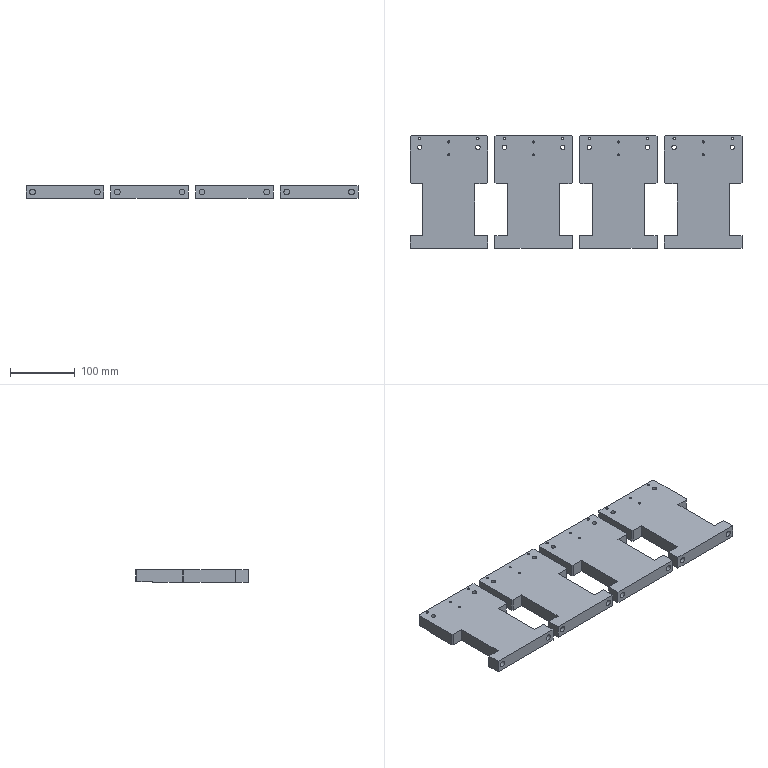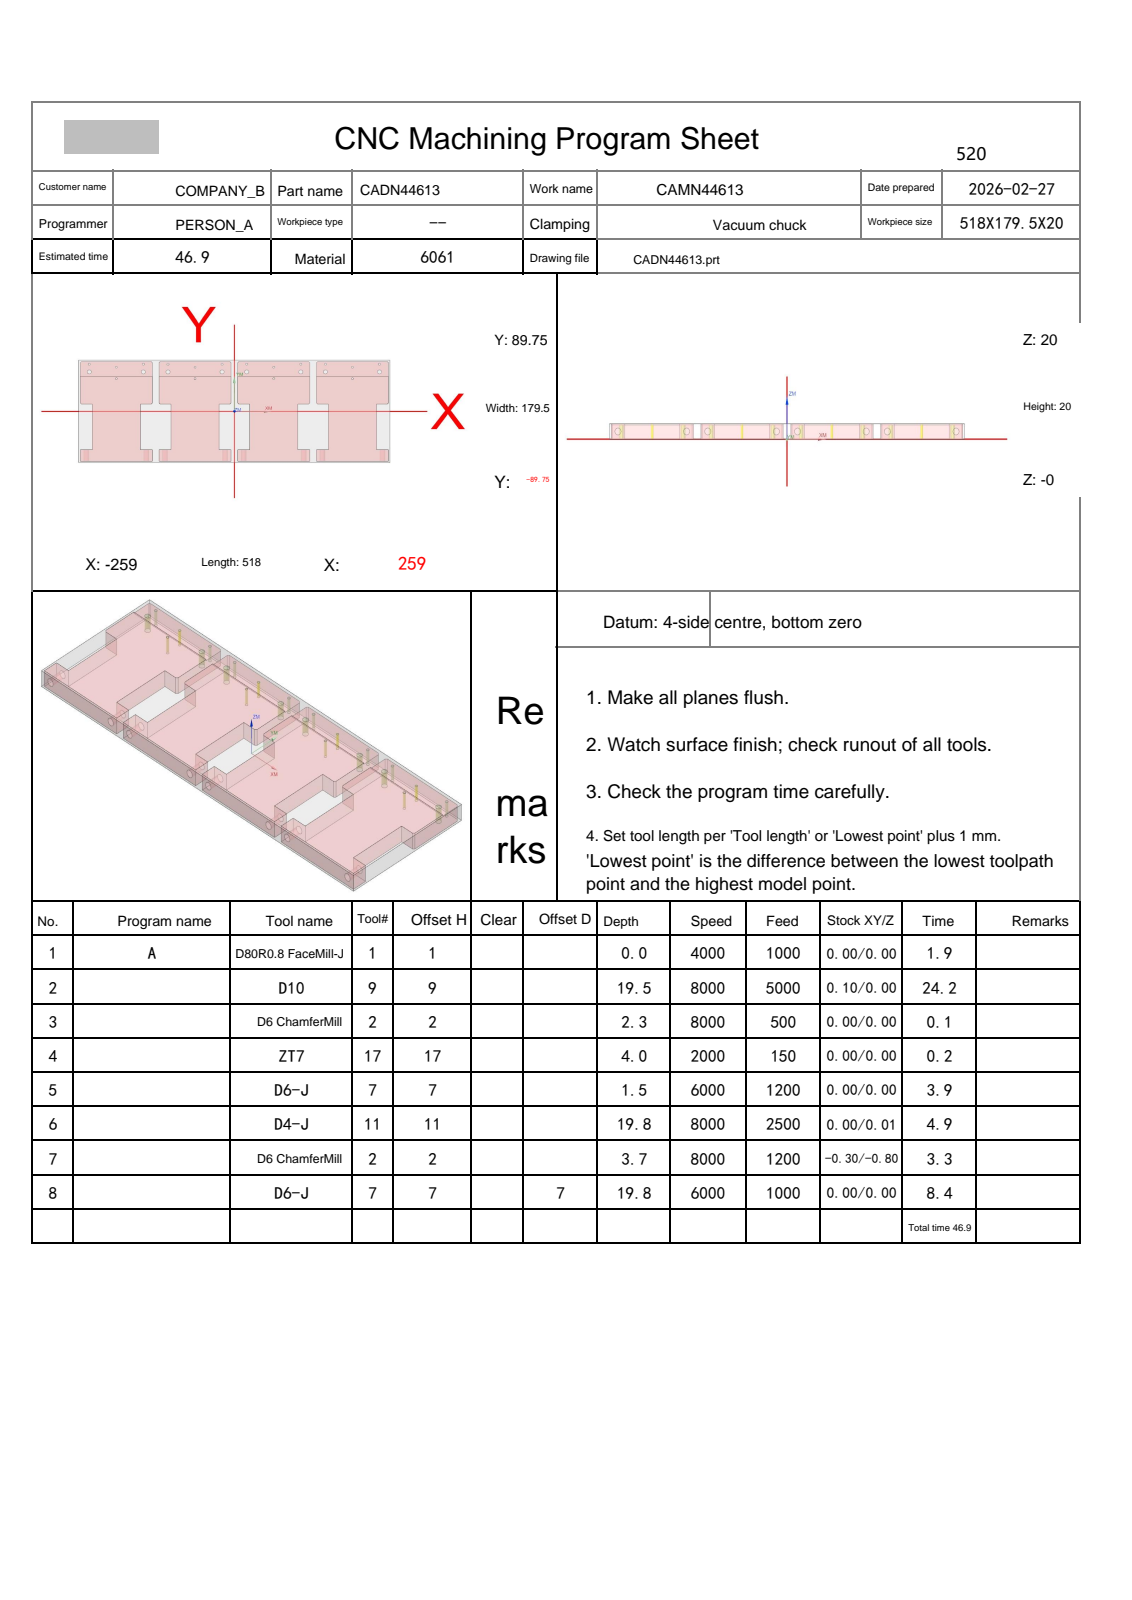NC program | NX | posted by the shop | part box 513 x 174.5 x 20 mm
Lines 41 to 1049 of 36838:
N2 T09 M06
(D10  D=10. R=0. H=09 ce=0.10 di=0.10)
G00 G90 G54 X-159.584 Y81.25 M03 S8000
G43 H09 Z50.
M08
Z20.5
G01 X-196.5 Z19.533 F4500.
X-250.5
Y73.2
X-142.5
Y81.25
X-196.5
Y88.25
X-254.914
X-257.5 Y85.664
Y66.2
X-135.5
Y85.664
X-138.086 Y88.25
X-196.5
X-197.
Z20.033
G00 Z20.5
X-159.584 Y81.25
Z20.033
G01 X-196.5 Z19.067
X-250.5
Y73.2
X-142.5
Y81.25
X-196.5
Y88.25
X-254.914
X-257.5 Y85.664
Y66.2
X-135.5
Y85.664
X-138.086 Y88.25
X-196.5
X-197.
Z19.567
G00 Z20.033
X-159.584 Y81.25
Z19.567
G01 X-196.5 Z18.6
X-250.5
Y73.2
X-142.5
Y81.25
X-196.5
Y88.25
X-254.914
X-257.5 Y85.664
Y66.2
X-135.5
Y85.664
X-138.086 Y88.25
X-196.5
X-197.
Z19.1
G00 Z50.
X-28.584 Y81.25
Z20.5
G01 X-65.5 Z19.533
X-119.5
Y73.2
X-11.5
Y81.25
X-65.5
Y88.25
X-123.914
X-126.5 Y85.664
Y66.2
X-4.5
Y85.664
X-7.086 Y88.25
X-65.5
X-66.
Z20.033
G00 Z20.5
X-28.584 Y81.25
Z20.033
G01 X-65.5 Z19.067
X-119.5
Y73.2
X-11.5
Y81.25
X-65.5
Y88.25
X-123.914
X-126.5 Y85.664
Y66.2
X-4.5
Y85.664
X-7.086 Y88.25
X-65.5
X-66.
Z19.567
G00 Z20.033
X-28.584 Y81.25
Z19.567
G01 X-65.5 Z18.6
X-119.5
Y73.2
X-11.5
Y81.25
X-65.5
Y88.25
X-123.914
X-126.5 Y85.664
Y66.2
X-4.5
Y85.664
X-7.086 Y88.25
X-65.5
X-66.
Z19.1
G00 Z50.
X102.416 Y81.25
Z20.5
G01 X65.5 Z19.533
X11.5
Y73.2
X119.5
Y81.25
X65.5
Y88.25
X7.086
X4.5 Y85.664
Y66.2
X126.5
Y85.664
X123.914 Y88.25
X65.5
X65.
Z20.033
G00 Z20.5
X102.416 Y81.25
Z20.033
G01 X65.5 Z19.067
X11.5
Y73.2
X119.5
Y81.25
X65.5
Y88.25
X7.086
X4.5 Y85.664
Y66.2
X126.5
Y85.664
X123.914 Y88.25
X65.5
X65.
Z19.567
G00 Z20.033
X102.416 Y81.25
Z19.567
G01 X65.5 Z18.6
X11.5
Y73.2
X119.5
Y81.25
X65.5
Y88.25
X7.086
X4.5 Y85.664
Y66.2
X126.5
Y85.664
X123.914 Y88.25
X65.5
X65.
Z19.1
G00 Z50.
X233.416 Y81.25
Z20.5
G01 X196.5 Z19.533
X142.5
Y73.2
X250.5
Y81.25
X196.5
Y88.25
X138.086
X135.5 Y85.664
Y66.2
X257.5
Y85.664
X254.914 Y88.25
X196.5
X196.
Z20.033
G00 Z20.5
X233.416 Y81.25
Z20.033
G01 X196.5 Z19.067
X142.5
Y73.2
X250.5
Y81.25
X196.5
Y88.25
X138.086
X135.5 Y85.664
Y66.2
X257.5
Y85.664
X254.914 Y88.25
X196.5
X196.
Z19.567
G00 Z20.033
X233.416 Y81.25
Z19.567
G01 X196.5 Z18.6
X142.5
Y73.2
X250.5
Y81.25
X196.5
Y88.25
X138.086
X135.5 Y85.664
Y66.2
X257.5
Y85.664
X254.914 Y88.25
X196.5
X196.
Z19.1
G00 Z50.
G00 G90 X196.5 Y-92.35 M03 S8000
Z50.
Z20.5
G01 X136.5 Z20.456 F5000.
G02 X131.4 Y-87.25 Z20.451 I0.0 J5.1
G01 Y-67.25 Z20.436
G02 X136.5 Y-62.15 Z20.43 I5.1 J0.0
G01 X151.4 Z20.419
Y7.65 Z20.369
X138.5 Z20.359
G02 X134.894 Y9.144 Z20.356 I0.0 J5.1
G01 X132.894 Y11.144 Z20.354
G02 X131.4 Y14.75 Z20.351 I3.606 J3.606
G01 Y85.25 Z20.3
G02 X132.894 Y88.856 Z20.297 I5.1 J0.0
G01 X134.894 Y90.856 Z20.295
G02 X138.5 Y92.35 Z20.292 I3.606 J-3.606
G01 X254.5 Z20.208
G02 X258.106 Y90.856 Z20.205 I0.0 J-5.1
G01 X260.106 Y88.856 Z20.203
G02 X261.6 Y85.25 Z20.2 I-3.606 J-3.606
G01 Y14.75 Z20.149
G02 X260.106 Y11.144 Z20.146 I-5.1 J0.0
G01 X258.106 Y9.144 Z20.144
G02 X254.5 Y7.65 Z20.141 I-3.606 J3.606
G01 X241.6 Z20.131
Y-62.15 Z20.081
X256.5 Z20.07
G02 X261.6 Y-67.25 Z20.064 I0.0 J-5.1
G01 Y-87.25 Z20.049
G02 X256.5 Y-92.35 Z20.044 I-5.1 J0.0
G01 X136.5 Z19.956
G02 X131.4 Y-87.25 Z19.951 I0.0 J5.1
G01 Y-67.25 Z19.936
G02 X136.5 Y-62.15 Z19.93 I5.1 J0.0
G01 X151.4 Z19.919
Y7.65 Z19.869
X138.5 Z19.859
G02 X134.894 Y9.144 Z19.856 I0.0 J5.1
G01 X132.894 Y11.144 Z19.854
G02 X131.4 Y14.75 Z19.851 I3.606 J3.606
G01 Y85.25 Z19.8
G02 X132.894 Y88.856 Z19.797 I5.1 J0.0
G01 X134.894 Y90.856 Z19.795
G02 X138.5 Y92.35 Z19.792 I3.606 J-3.606
G01 X254.5 Z19.708
G02 X258.106 Y90.856 Z19.705 I0.0 J-5.1
G01 X260.106 Y88.856 Z19.703
G02 X261.6 Y85.25 Z19.7 I-3.606 J-3.606
G01 Y14.75 Z19.649
G02 X260.106 Y11.144 Z19.646 I-5.1 J0.0
G01 X258.106 Y9.144 Z19.644
G02 X254.5 Y7.65 Z19.641 I-3.606 J3.606
G01 X241.6 Z19.631
Y-62.15 Z19.581
X256.5 Z19.57
G02 X261.6 Y-67.25 Z19.564 I0.0 J-5.1
G01 Y-87.25 Z19.549
G02 X256.5 Y-92.35 Z19.544 I-5.1 J0.0
G01 X136.5 Z19.456
G02 X131.4 Y-87.25 Z19.451 I0.0 J5.1
G01 Y-67.25 Z19.436
G02 X136.5 Y-62.15 Z19.43 I5.1 J0.0
G01 X151.4 Z19.419
Y7.65 Z19.369
X138.5 Z19.359
G02 X134.894 Y9.144 Z19.356 I0.0 J5.1
G01 X132.894 Y11.144 Z19.354
G02 X131.4 Y14.75 Z19.351 I3.606 J3.606
G01 Y85.25 Z19.3
G02 X132.894 Y88.856 Z19.297 I5.1 J0.0
G01 X134.894 Y90.856 Z19.295
G02 X138.5 Y92.35 Z19.292 I3.606 J-3.606
G01 X254.5 Z19.208
G02 X258.106 Y90.856 Z19.205 I0.0 J-5.1
G01 X260.106 Y88.856 Z19.203
G02 X261.6 Y85.25 Z19.2 I-3.606 J-3.606
G01 Y14.75 Z19.149
G02 X260.106 Y11.144 Z19.146 I-5.1 J0.0
G01 X258.106 Y9.144 Z19.144
G02 X254.5 Y7.65 Z19.141 I-3.606 J3.606
G01 X241.6 Z19.131
Y-62.15 Z19.081
X256.5 Z19.07
G02 X261.6 Y-67.25 Z19.064 I0.0 J-5.1
G01 Y-87.25 Z19.049
G02 X256.5 Y-92.35 Z19.044 I-5.1 J0.0
G01 X136.5 Z18.956
G02 X131.4 Y-87.25 Z18.951 I0.0 J5.1
G01 Y-67.25 Z18.936
G02 X136.5 Y-62.15 Z18.93 I5.1 J0.0
G01 X151.4 Z18.919
Y7.65 Z18.869
X138.5 Z18.859
G02 X134.894 Y9.144 Z18.856 I0.0 J5.1
G01 X132.894 Y11.144 Z18.854
G02 X131.4 Y14.75 Z18.851 I3.606 J3.606
G01 Y85.25 Z18.8
G02 X132.894 Y88.856 Z18.797 I5.1 J0.0
G01 X134.894 Y90.856 Z18.795
G02 X138.5 Y92.35 Z18.792 I3.606 J-3.606
G01 X254.5 Z18.708
G02 X258.106 Y90.856 Z18.705 I0.0 J-5.1
G01 X260.106 Y88.856 Z18.703
G02 X261.6 Y85.25 Z18.7 I-3.606 J-3.606
G01 Y14.75 Z18.649
G02 X260.106 Y11.144 Z18.646 I-5.1 J0.0
G01 X258.106 Y9.144 Z18.644
G02 X254.5 Y7.65 Z18.641 I-3.606 J3.606
G01 X241.6 Z18.631
Y-62.15 Z18.581
X256.5 Z18.57
G02 X261.6 Y-67.25 Z18.564 I0.0 J-5.1
G01 Y-87.25 Z18.549
G02 X256.5 Y-92.35 Z18.544 I-5.1 J0.0
G01 X136.5 Z18.456
G02 X131.4 Y-87.25 Z18.451 I0.0 J5.1
G01 Y-67.25 Z18.436
G02 X136.5 Y-62.15 Z18.43 I5.1 J0.0
G01 X151.4 Z18.419
Y7.65 Z18.369
X138.5 Z18.359
G02 X134.894 Y9.144 Z18.356 I0.0 J5.1
G01 X132.894 Y11.144 Z18.354
G02 X131.4 Y14.75 Z18.351 I3.606 J3.606
G01 Y85.25 Z18.3
G02 X132.894 Y88.856 Z18.297 I5.1 J0.0
G01 X134.894 Y90.856 Z18.295
G02 X138.5 Y92.35 Z18.292 I3.606 J-3.606
G01 X254.5 Z18.208
G02 X258.106 Y90.856 Z18.205 I0.0 J-5.1
G01 X260.106 Y88.856 Z18.203
G02 X261.6 Y85.25 Z18.2 I-3.606 J-3.606
G01 Y14.75 Z18.149
G02 X260.106 Y11.144 Z18.146 I-5.1 J0.0
G01 X258.106 Y9.144 Z18.144
G02 X254.5 Y7.65 Z18.141 I-3.606 J3.606
G01 X241.6 Z18.131
Y-62.15 Z18.081
X256.5 Z18.07
G02 X261.6 Y-67.25 Z18.064 I0.0 J-5.1
G01 Y-87.25 Z18.049
G02 X256.5 Y-92.35 Z18.044 I-5.1 J0.0
G01 X136.5 Z17.956
G02 X131.4 Y-87.25 Z17.951 I0.0 J5.1
G01 Y-67.25 Z17.936
G02 X136.5 Y-62.15 Z17.93 I5.1 J0.0
G01 X151.4 Z17.919
Y7.65 Z17.869
X138.5 Z17.859
G02 X134.894 Y9.144 Z17.856 I0.0 J5.1
G01 X132.894 Y11.144 Z17.854
G02 X131.4 Y14.75 Z17.851 I3.606 J3.606
G01 Y85.25 Z17.8
G02 X132.894 Y88.856 Z17.797 I5.1 J0.0
G01 X134.894 Y90.856 Z17.795
G02 X138.5 Y92.35 Z17.792 I3.606 J-3.606
G01 X254.5 Z17.708
G02 X258.106 Y90.856 Z17.705 I0.0 J-5.1
G01 X260.106 Y88.856 Z17.703
G02 X261.6 Y85.25 Z17.7 I-3.606 J-3.606
G01 Y14.75 Z17.649
G02 X260.106 Y11.144 Z17.646 I-5.1 J0.0
G01 X258.106 Y9.144 Z17.644
G02 X254.5 Y7.65 Z17.641 I-3.606 J3.606
G01 X241.6 Z17.631
Y-62.15 Z17.581
X256.5 Z17.57
G02 X261.6 Y-67.25 Z17.564 I0.0 J-5.1
G01 Y-87.25 Z17.549
G02 X256.5 Y-92.35 Z17.544 I-5.1 J0.0
G01 X136.5 Z17.456
G02 X131.4 Y-87.25 Z17.451 I0.0 J5.1
G01 Y-67.25 Z17.436
G02 X136.5 Y-62.15 Z17.43 I5.1 J0.0
G01 X151.4 Z17.419
Y7.65 Z17.369
X138.5 Z17.359
G02 X134.894 Y9.144 Z17.356 I0.0 J5.1
G01 X132.894 Y11.144 Z17.354
G02 X131.4 Y14.75 Z17.351 I3.606 J3.606
G01 Y85.25 Z17.3
G02 X132.894 Y88.856 Z17.297 I5.1 J0.0
G01 X134.894 Y90.856 Z17.295
G02 X138.5 Y92.35 Z17.292 I3.606 J-3.606
G01 X254.5 Z17.208
G02 X258.106 Y90.856 Z17.205 I0.0 J-5.1
G01 X260.106 Y88.856 Z17.203
G02 X261.6 Y85.25 Z17.2 I-3.606 J-3.606
G01 Y14.75 Z17.149
G02 X260.106 Y11.144 Z17.146 I-5.1 J0.0
G01 X258.106 Y9.144 Z17.144
G02 X254.5 Y7.65 Z17.141 I-3.606 J3.606
G01 X241.6 Z17.131
Y-62.15 Z17.081
X256.5 Z17.07
G02 X261.6 Y-67.25 Z17.064 I0.0 J-5.1
G01 Y-87.25 Z17.049
G02 X256.5 Y-92.35 Z17.044 I-5.1 J0.0
G01 X136.5 Z16.956
G02 X131.4 Y-87.25 Z16.951 I0.0 J5.1
G01 Y-67.25 Z16.936
G02 X136.5 Y-62.15 Z16.93 I5.1 J0.0
G01 X151.4 Z16.919
Y7.65 Z16.869
X138.5 Z16.859
G02 X134.894 Y9.144 Z16.856 I0.0 J5.1
G01 X132.894 Y11.144 Z16.854
G02 X131.4 Y14.75 Z16.851 I3.606 J3.606
G01 Y85.25 Z16.8
G02 X132.894 Y88.856 Z16.797 I5.1 J0.0
G01 X134.894 Y90.856 Z16.795
G02 X138.5 Y92.35 Z16.792 I3.606 J-3.606
G01 X254.5 Z16.708
G02 X258.106 Y90.856 Z16.705 I0.0 J-5.1
G01 X260.106 Y88.856 Z16.703
G02 X261.6 Y85.25 Z16.7 I-3.606 J-3.606
G01 Y14.75 Z16.649
G02 X260.106 Y11.144 Z16.646 I-5.1 J0.0
G01 X258.106 Y9.144 Z16.644
G02 X254.5 Y7.65 Z16.641 I-3.606 J3.606
G01 X241.6 Z16.631
Y-62.15 Z16.581
X256.5 Z16.57
G02 X261.6 Y-67.25 Z16.564 I0.0 J-5.1
G01 Y-87.25 Z16.549
G02 X256.5 Y-92.35 Z16.544 I-5.1 J0.0
G01 X136.5 Z16.456
G02 X131.4 Y-87.25 Z16.451 I0.0 J5.1
G01 Y-67.25 Z16.436
G02 X136.5 Y-62.15 Z16.43 I5.1 J0.0
G01 X151.4 Z16.419
Y7.65 Z16.369
X138.5 Z16.359
G02 X134.894 Y9.144 Z16.356 I0.0 J5.1
G01 X132.894 Y11.144 Z16.354
G02 X131.4 Y14.75 Z16.351 I3.606 J3.606
G01 Y85.25 Z16.3
G02 X132.894 Y88.856 Z16.297 I5.1 J0.0
G01 X134.894 Y90.856 Z16.295
G02 X138.5 Y92.35 Z16.292 I3.606 J-3.606
G01 X254.5 Z16.208
G02 X258.106 Y90.856 Z16.205 I0.0 J-5.1
G01 X260.106 Y88.856 Z16.203
G02 X261.6 Y85.25 Z16.2 I-3.606 J-3.606
G01 Y14.75 Z16.149
G02 X260.106 Y11.144 Z16.146 I-5.1 J0.0
G01 X258.106 Y9.144 Z16.144
G02 X254.5 Y7.65 Z16.141 I-3.606 J3.606
G01 X241.6 Z16.131
Y-62.15 Z16.081
X256.5 Z16.07
G02 X261.6 Y-67.25 Z16.064 I0.0 J-5.1
G01 Y-87.25 Z16.049
G02 X256.5 Y-92.35 Z16.044 I-5.1 J0.0
G01 X136.5 Z15.956
G02 X131.4 Y-87.25 Z15.951 I0.0 J5.1
G01 Y-67.25 Z15.936
G02 X136.5 Y-62.15 Z15.93 I5.1 J0.0
G01 X151.4 Z15.919
Y7.65 Z15.869
X138.5 Z15.859
G02 X134.894 Y9.144 Z15.856 I0.0 J5.1
G01 X132.894 Y11.144 Z15.854
G02 X131.4 Y14.75 Z15.851 I3.606 J3.606
G01 Y85.25 Z15.8
G02 X132.894 Y88.856 Z15.797 I5.1 J0.0
G01 X134.894 Y90.856 Z15.795
G02 X138.5 Y92.35 Z15.792 I3.606 J-3.606
G01 X254.5 Z15.708
G02 X258.106 Y90.856 Z15.705 I0.0 J-5.1
G01 X260.106 Y88.856 Z15.703
G02 X261.6 Y85.25 Z15.7 I-3.606 J-3.606
G01 Y14.75 Z15.649
G02 X260.106 Y11.144 Z15.646 I-5.1 J0.0
G01 X258.106 Y9.144 Z15.644
G02 X254.5 Y7.65 Z15.641 I-3.606 J3.606
G01 X241.6 Z15.631
Y-62.15 Z15.581
X256.5 Z15.57
G02 X261.6 Y-67.25 Z15.564 I0.0 J-5.1
G01 Y-87.25 Z15.549
G02 X256.5 Y-92.35 Z15.544 I-5.1 J0.0
G01 X136.5 Z15.456
G02 X131.4 Y-87.25 Z15.451 I0.0 J5.1
G01 Y-67.25 Z15.436
G02 X136.5 Y-62.15 Z15.43 I5.1 J0.0
G01 X151.4 Z15.419
Y7.65 Z15.369
X138.5 Z15.359
G02 X134.894 Y9.144 Z15.356 I0.0 J5.1
G01 X132.894 Y11.144 Z15.354
G02 X131.4 Y14.75 Z15.351 I3.606 J3.606
G01 Y85.25 Z15.3
G02 X132.894 Y88.856 Z15.297 I5.1 J0.0
G01 X134.894 Y90.856 Z15.295
G02 X138.5 Y92.35 Z15.292 I3.606 J-3.606
G01 X254.5 Z15.208
G02 X258.106 Y90.856 Z15.205 I0.0 J-5.1
G01 X260.106 Y88.856 Z15.203
G02 X261.6 Y85.25 Z15.2 I-3.606 J-3.606
G01 Y14.75 Z15.149
G02 X260.106 Y11.144 Z15.146 I-5.1 J0.0
G01 X258.106 Y9.144 Z15.144
G02 X254.5 Y7.65 Z15.141 I-3.606 J3.606
G01 X241.6 Z15.131
Y-62.15 Z15.081
X256.5 Z15.07
G02 X261.6 Y-67.25 Z15.064 I0.0 J-5.1
G01 Y-87.25 Z15.049
G02 X256.5 Y-92.35 Z15.044 I-5.1 J0.0
G01 X136.5 Z14.956
G02 X131.4 Y-87.25 Z14.951 I0.0 J5.1
G01 Y-67.25 Z14.936
G02 X136.5 Y-62.15 Z14.93 I5.1 J0.0
G01 X151.4 Z14.919
Y7.65 Z14.869
X138.5 Z14.859
G02 X134.894 Y9.144 Z14.856 I0.0 J5.1
G01 X132.894 Y11.144 Z14.854
G02 X131.4 Y14.75 Z14.851 I3.606 J3.606
G01 Y85.25 Z14.8
G02 X132.894 Y88.856 Z14.797 I5.1 J0.0
G01 X134.894 Y90.856 Z14.795
G02 X138.5 Y92.35 Z14.792 I3.606 J-3.606
G01 X254.5 Z14.708
G02 X258.106 Y90.856 Z14.705 I0.0 J-5.1
G01 X260.106 Y88.856 Z14.703
G02 X261.6 Y85.25 Z14.7 I-3.606 J-3.606
G01 Y14.75 Z14.649
G02 X260.106 Y11.144 Z14.646 I-5.1 J0.0
G01 X258.106 Y9.144 Z14.644
G02 X254.5 Y7.65 Z14.641 I-3.606 J3.606
G01 X241.6 Z14.631
Y-62.15 Z14.581
X256.5 Z14.57
G02 X261.6 Y-67.25 Z14.564 I0.0 J-5.1
G01 Y-87.25 Z14.549
G02 X256.5 Y-92.35 Z14.544 I-5.1 J0.0
G01 X136.5 Z14.456
G02 X131.4 Y-87.25 Z14.451 I0.0 J5.1
G01 Y-67.25 Z14.436
G02 X136.5 Y-62.15 Z14.43 I5.1 J0.0
G01 X151.4 Z14.419
Y7.65 Z14.369
X138.5 Z14.359
G02 X134.894 Y9.144 Z14.356 I0.0 J5.1
G01 X132.894 Y11.144 Z14.354
G02 X131.4 Y14.75 Z14.351 I3.606 J3.606
G01 Y85.25 Z14.3
G02 X132.894 Y88.856 Z14.297 I5.1 J0.0
G01 X134.894 Y90.856 Z14.295
G02 X138.5 Y92.35 Z14.292 I3.606 J-3.606
G01 X254.5 Z14.208
G02 X258.106 Y90.856 Z14.205 I0.0 J-5.1
G01 X260.106 Y88.856 Z14.203
G02 X261.6 Y85.25 Z14.2 I-3.606 J-3.606
G01 Y14.75 Z14.149
G02 X260.106 Y11.144 Z14.146 I-5.1 J0.0
G01 X258.106 Y9.144 Z14.144
G02 X254.5 Y7.65 Z14.141 I-3.606 J3.606
G01 X241.6 Z14.131
Y-62.15 Z14.081
X256.5 Z14.07
G02 X261.6 Y-67.25 Z14.064 I0.0 J-5.1
G01 Y-87.25 Z14.049
G02 X256.5 Y-92.35 Z14.044 I-5.1 J0.0
G01 X136.5 Z13.956
G02 X131.4 Y-87.25 Z13.951 I0.0 J5.1
G01 Y-67.25 Z13.936
G02 X136.5 Y-62.15 Z13.93 I5.1 J0.0
G01 X151.4 Z13.919
Y7.65 Z13.869
X138.5 Z13.859
G02 X134.894 Y9.144 Z13.856 I0.0 J5.1
G01 X132.894 Y11.144 Z13.854
G02 X131.4 Y14.75 Z13.851 I3.606 J3.606
G01 Y85.25 Z13.8
G02 X132.894 Y88.856 Z13.797 I5.1 J0.0
G01 X134.894 Y90.856 Z13.795
G02 X138.5 Y92.35 Z13.792 I3.606 J-3.606
G01 X254.5 Z13.708
G02 X258.106 Y90.856 Z13.705 I0.0 J-5.1
G01 X260.106 Y88.856 Z13.703
G02 X261.6 Y85.25 Z13.7 I-3.606 J-3.606
G01 Y14.75 Z13.649
G02 X260.106 Y11.144 Z13.646 I-5.1 J0.0
G01 X258.106 Y9.144 Z13.644
G02 X254.5 Y7.65 Z13.641 I-3.606 J3.606
G01 X241.6 Z13.631
Y-62.15 Z13.581
X256.5 Z13.57
G02 X261.6 Y-67.25 Z13.564 I0.0 J-5.1
G01 Y-87.25 Z13.549
G02 X256.5 Y-92.35 Z13.544 I-5.1 J0.0
G01 X136.5 Z13.456
G02 X131.4 Y-87.25 Z13.451 I0.0 J5.1
G01 Y-67.25 Z13.436
G02 X136.5 Y-62.15 Z13.43 I5.1 J0.0
G01 X151.4 Z13.419
Y7.65 Z13.369
X138.5 Z13.359
G02 X134.894 Y9.144 Z13.356 I0.0 J5.1
G01 X132.894 Y11.144 Z13.354
G02 X131.4 Y14.75 Z13.351 I3.606 J3.606
G01 Y85.25 Z13.3
G02 X132.894 Y88.856 Z13.297 I5.1 J0.0
G01 X134.894 Y90.856 Z13.295
G02 X138.5 Y92.35 Z13.292 I3.606 J-3.606
G01 X254.5 Z13.208
G02 X258.106 Y90.856 Z13.205 I0.0 J-5.1
G01 X260.106 Y88.856 Z13.203
G02 X261.6 Y85.25 Z13.2 I-3.606 J-3.606
G01 Y14.75 Z13.149
G02 X260.106 Y11.144 Z13.146 I-5.1 J0.0
G01 X258.106 Y9.144 Z13.144
G02 X254.5 Y7.65 Z13.141 I-3.606 J3.606
G01 X241.6 Z13.131
Y-62.15 Z13.081
X256.5 Z13.07
G02 X261.6 Y-67.25 Z13.064 I0.0 J-5.1
G01 Y-87.25 Z13.049
G02 X256.5 Y-92.35 Z13.044 I-5.1 J0.0
G01 X136.5 Z12.956
G02 X131.4 Y-87.25 Z12.951 I0.0 J5.1
G01 Y-67.25 Z12.936
G02 X136.5 Y-62.15 Z12.93 I5.1 J0.0
G01 X151.4 Z12.919
Y7.65 Z12.869
X138.5 Z12.859
G02 X134.894 Y9.144 Z12.856 I0.0 J5.1
G01 X132.894 Y11.144 Z12.854
G02 X131.4 Y14.75 Z12.851 I3.606 J3.606
G01 Y85.25 Z12.8
G02 X132.894 Y88.856 Z12.797 I5.1 J0.0
G01 X134.894 Y90.856 Z12.795
G02 X138.5 Y92.35 Z12.792 I3.606 J-3.606
G01 X254.5 Z12.708
G02 X258.106 Y90.856 Z12.705 I0.0 J-5.1
G01 X260.106 Y88.856 Z12.703
G02 X261.6 Y85.25 Z12.7 I-3.606 J-3.606
G01 Y14.75 Z12.649
G02 X260.106 Y11.144 Z12.646 I-5.1 J0.0
G01 X258.106 Y9.144 Z12.644
G02 X254.5 Y7.65 Z12.641 I-3.606 J3.606
G01 X241.6 Z12.631
Y-62.15 Z12.581
X256.5 Z12.57
G02 X261.6 Y-67.25 Z12.564 I0.0 J-5.1
G01 Y-87.25 Z12.549
G02 X256.5 Y-92.35 Z12.544 I-5.1 J0.0
G01 X136.5 Z12.456
G02 X131.4 Y-87.25 Z12.451 I0.0 J5.1
G01 Y-67.25 Z12.436
G02 X136.5 Y-62.15 Z12.43 I5.1 J0.0
G01 X151.4 Z12.419
Y7.65 Z12.369
X138.5 Z12.359
G02 X134.894 Y9.144 Z12.356 I0.0 J5.1
G01 X132.894 Y11.144 Z12.354
G02 X131.4 Y14.75 Z12.351 I3.606 J3.606
G01 Y85.25 Z12.3
G02 X132.894 Y88.856 Z12.297 I5.1 J0.0
G01 X134.894 Y90.856 Z12.295
G02 X138.5 Y92.35 Z12.292 I3.606 J-3.606
G01 X254.5 Z12.208
G02 X258.106 Y90.856 Z12.205 I0.0 J-5.1
G01 X260.106 Y88.856 Z12.203
G02 X261.6 Y85.25 Z12.2 I-3.606 J-3.606
G01 Y14.75 Z12.149
G02 X260.106 Y11.144 Z12.146 I-5.1 J0.0
G01 X258.106 Y9.144 Z12.144
G02 X254.5 Y7.65 Z12.141 I-3.606 J3.606
G01 X241.6 Z12.131
Y-62.15 Z12.081
X256.5 Z12.07
G02 X261.6 Y-67.25 Z12.064 I0.0 J-5.1
G01 Y-87.25 Z12.049
G02 X256.5 Y-92.35 Z12.044 I-5.1 J0.0
G01 X136.5 Z11.956
G02 X131.4 Y-87.25 Z11.951 I0.0 J5.1
G01 Y-67.25 Z11.936
G02 X136.5 Y-62.15 Z11.93 I5.1 J0.0
G01 X151.4 Z11.919
Y7.65 Z11.869
X138.5 Z11.859
G02 X134.894 Y9.144 Z11.856 I0.0 J5.1
G01 X132.894 Y11.144 Z11.854
G02 X131.4 Y14.75 Z11.851 I3.606 J3.606
G01 Y85.25 Z11.8
G02 X132.894 Y88.856 Z11.797 I5.1 J0.0
G01 X134.894 Y90.856 Z11.795
G02 X138.5 Y92.35 Z11.792 I3.606 J-3.606
G01 X254.5 Z11.708
G02 X258.106 Y90.856 Z11.705 I0.0 J-5.1
G01 X260.106 Y88.856 Z11.703
G02 X261.6 Y85.25 Z11.7 I-3.606 J-3.606
G01 Y14.75 Z11.649
G02 X260.106 Y11.144 Z11.646 I-5.1 J0.0
G01 X258.106 Y9.144 Z11.644
G02 X254.5 Y7.65 Z11.641 I-3.606 J3.606
G01 X241.6 Z11.631
Y-62.15 Z11.581
X256.5 Z11.57
G02 X261.6 Y-67.25 Z11.564 I0.0 J-5.1
G01 Y-87.25 Z11.549
G02 X256.5 Y-92.35 Z11.544 I-5.1 J0.0
G01 X136.5 Z11.456
G02 X131.4 Y-87.25 Z11.451 I0.0 J5.1
G01 Y-67.25 Z11.436
G02 X136.5 Y-62.15 Z11.43 I5.1 J0.0
G01 X151.4 Z11.419
Y7.65 Z11.369
X138.5 Z11.359
G02 X134.894 Y9.144 Z11.356 I0.0 J5.1
G01 X132.894 Y11.144 Z11.354
G02 X131.4 Y14.75 Z11.351 I3.606 J3.606
G01 Y85.25 Z11.3
G02 X132.894 Y88.856 Z11.297 I5.1 J0.0
G01 X134.894 Y90.856 Z11.295
G02 X138.5 Y92.35 Z11.292 I3.606 J-3.606
G01 X254.5 Z11.208
G02 X258.106 Y90.856 Z11.205 I0.0 J-5.1
G01 X260.106 Y88.856 Z11.203
G02 X261.6 Y85.25 Z11.2 I-3.606 J-3.606
G01 Y14.75 Z11.149
G02 X260.106 Y11.144 Z11.146 I-5.1 J0.0
G01 X258.106 Y9.144 Z11.144
G02 X254.5 Y7.65 Z11.141 I-3.606 J3.606
G01 X241.6 Z11.131
Y-62.15 Z11.081
X256.5 Z11.07
G02 X261.6 Y-67.25 Z11.064 I0.0 J-5.1
G01 Y-87.25 Z11.049
G02 X256.5 Y-92.35 Z11.044 I-5.1 J0.0
G01 X136.5 Z10.956
G02 X131.4 Y-87.25 Z10.951 I0.0 J5.1
G01 Y-67.25 Z10.936
G02 X136.5 Y-62.15 Z10.93 I5.1 J0.0
G01 X151.4 Z10.919
Y7.65 Z10.869
X138.5 Z10.859
G02 X134.894 Y9.144 Z10.856 I0.0 J5.1
G01 X132.894 Y11.144 Z10.854
G02 X131.4 Y14.75 Z10.851 I3.606 J3.606
G01 Y85.25 Z10.8
G02 X132.894 Y88.856 Z10.797 I5.1 J0.0
G01 X134.894 Y90.856 Z10.795
G02 X138.5 Y92.35 Z10.792 I3.606 J-3.606
G01 X254.5 Z10.708
G02 X258.106 Y90.856 Z10.705 I0.0 J-5.1
G01 X260.106 Y88.856 Z10.703
G02 X261.6 Y85.25 Z10.7 I-3.606 J-3.606
G01 Y14.75 Z10.649
G02 X260.106 Y11.144 Z10.646 I-5.1 J0.0
G01 X258.106 Y9.144 Z10.644
G02 X254.5 Y7.65 Z10.641 I-3.606 J3.606
G01 X241.6 Z10.631
Y-62.15 Z10.581
X256.5 Z10.57
G02 X261.6 Y-67.25 Z10.564 I0.0 J-5.1
G01 Y-87.25 Z10.549
G02 X256.5 Y-92.35 Z10.544 I-5.1 J0.0
G01 X136.5 Z10.456
G02 X131.4 Y-87.25 Z10.451 I0.0 J5.1
G01 Y-67.25 Z10.436
G02 X136.5 Y-62.15 Z10.43 I5.1 J0.0
G01 X151.4 Z10.419
Y7.65 Z10.369
X138.5 Z10.359
G02 X134.894 Y9.144 Z10.356 I0.0 J5.1
G01 X132.894 Y11.144 Z10.354
G02 X131.4 Y14.75 Z10.351 I3.606 J3.606
G01 Y85.25 Z10.3
G02 X132.894 Y88.856 Z10.297 I5.1 J0.0
G01 X134.894 Y90.856 Z10.295
G02 X138.5 Y92.35 Z10.292 I3.606 J-3.606
G01 X254.5 Z10.208
G02 X258.106 Y90.856 Z10.205 I0.0 J-5.1
G01 X260.106 Y88.856 Z10.203
G02 X261.6 Y85.25 Z10.2 I-3.606 J-3.606
G01 Y14.75 Z10.149
G02 X260.106 Y11.144 Z10.146 I-5.1 J0.0
G01 X258.106 Y9.144 Z10.144
G02 X254.5 Y7.65 Z10.141 I-3.606 J3.606
G01 X241.6 Z10.131
Y-62.15 Z10.081
X256.5 Z10.07
G02 X261.6 Y-67.25 Z10.064 I0.0 J-5.1
G01 Y-87.25 Z10.049
G02 X256.5 Y-92.35 Z10.044 I-5.1 J0.0
G01 X136.5 Z9.956
G02 X131.4 Y-87.25 Z9.951 I0.0 J5.1
G01 Y-67.25 Z9.936
G02 X136.5 Y-62.15 Z9.93 I5.1 J0.0
G01 X151.4 Z9.919
Y7.65 Z9.869
X138.5 Z9.859
G02 X134.894 Y9.144 Z9.856 I0.0 J5.1
G01 X132.894 Y11.144 Z9.854
G02 X131.4 Y14.75 Z9.851 I3.606 J3.606
G01 Y85.25 Z9.8
G02 X132.894 Y88.856 Z9.797 I5.1 J0.0
G01 X134.894 Y90.856 Z9.795
G02 X138.5 Y92.35 Z9.792 I3.606 J-3.606
G01 X254.5 Z9.708
G02 X258.106 Y90.856 Z9.705 I0.0 J-5.1
G01 X260.106 Y88.856 Z9.703
G02 X261.6 Y85.25 Z9.7 I-3.606 J-3.606
G01 Y14.75 Z9.649
G02 X260.106 Y11.144 Z9.646 I-5.1 J0.0
G01 X258.106 Y9.144 Z9.644
G02 X254.5 Y7.65 Z9.641 I-3.606 J3.606
G01 X241.6 Z9.631
Y-62.15 Z9.581
X256.5 Z9.57
G02 X261.6 Y-67.25 Z9.564 I0.0 J-5.1
G01 Y-87.25 Z9.549
G02 X256.5 Y-92.35 Z9.544 I-5.1 J0.0
G01 X136.5 Z9.456
G02 X131.4 Y-87.25 Z9.451 I0.0 J5.1
G01 Y-67.25 Z9.436
G02 X136.5 Y-62.15 Z9.43 I5.1 J0.0
G01 X151.4 Z9.419
Y7.65 Z9.369
X138.5 Z9.359
G02 X134.894 Y9.144 Z9.356 I0.0 J5.1
G01 X132.894 Y11.144 Z9.354
G02 X131.4 Y14.75 Z9.351 I3.606 J3.606
G01 Y85.25 Z9.3
G02 X132.894 Y88.856 Z9.297 I5.1 J0.0
G01 X134.894 Y90.856 Z9.295
G02 X138.5 Y92.35 Z9.292 I3.606 J-3.606
G01 X254.5 Z9.208
G02 X258.106 Y90.856 Z9.205 I0.0 J-5.1
G01 X260.106 Y88.856 Z9.203
G02 X261.6 Y85.25 Z9.2 I-3.606 J-3.606
G01 Y14.75 Z9.149
G02 X260.106 Y11.144 Z9.146 I-5.1 J0.0
G01 X258.106 Y9.144 Z9.144
G02 X254.5 Y7.65 Z9.141 I-3.606 J3.606
G01 X241.6 Z9.131
Y-62.15 Z9.081
X256.5 Z9.07
G02 X261.6 Y-67.25 Z9.064 I0.0 J-5.1
G01 Y-87.25 Z9.049
G02 X256.5 Y-92.35 Z9.044 I-5.1 J0.0
G01 X136.5 Z8.956
G02 X131.4 Y-87.25 Z8.951 I0.0 J5.1
G01 Y-67.25 Z8.936
G02 X136.5 Y-62.15 Z8.93 I5.1 J0.0
G01 X151.4 Z8.919
Y7.65 Z8.869
X138.5 Z8.859
G02 X134.894 Y9.144 Z8.856 I0.0 J5.1
G01 X132.894 Y11.144 Z8.854
G02 X131.4 Y14.75 Z8.851 I3.606 J3.606
G01 Y85.25 Z8.8
G02 X132.894 Y88.856 Z8.797 I5.1 J0.0
G01 X134.894 Y90.856 Z8.795
G02 X138.5 Y92.35 Z8.792 I3.606 J-3.606
G01 X254.5 Z8.708
G02 X258.106 Y90.856 Z8.705 I0.0 J-5.1
G01 X260.106 Y88.856 Z8.703
G02 X261.6 Y85.25 Z8.7 I-3.606 J-3.606
G01 Y14.75 Z8.649
G02 X260.106 Y11.144 Z8.646 I-5.1 J0.0
G01 X258.106 Y9.144 Z8.644
G02 X254.5 Y7.65 Z8.641 I-3.606 J3.606
G01 X241.6 Z8.631
Y-62.15 Z8.581
X256.5 Z8.57
G02 X261.6 Y-67.25 Z8.564 I0.0 J-5.1
G01 Y-87.25 Z8.549
G02 X256.5 Y-92.35 Z8.544 I-5.1 J0.0
G01 X136.5 Z8.456
G02 X131.4 Y-87.25 Z8.451 I0.0 J5.1
G01 Y-67.25 Z8.436
G02 X136.5 Y-62.15 Z8.43 I5.1 J0.0
G01 X151.4 Z8.419
Y7.65 Z8.369
X138.5 Z8.359
G02 X134.894 Y9.144 Z8.356 I0.0 J5.1
G01 X132.894 Y11.144 Z8.354
G02 X131.4 Y14.75 Z8.351 I3.606 J3.606
G01 Y85.25 Z8.3
G02 X132.894 Y88.856 Z8.297 I5.1 J0.0
G01 X134.894 Y90.856 Z8.295
G02 X138.5 Y92.35 Z8.292 I3.606 J-3.606
G01 X254.5 Z8.208
G02 X258.106 Y90.856 Z8.205 I0.0 J-5.1
G01 X260.106 Y88.856 Z8.203
G02 X261.6 Y85.25 Z8.2 I-3.606 J-3.606
G01 Y14.75 Z8.149
G02 X260.106 Y11.144 Z8.146 I-5.1 J0.0
G01 X258.106 Y9.144 Z8.144
G02 X254.5 Y7.65 Z8.141 I-3.606 J3.606
G01 X241.6 Z8.131
Y-62.15 Z8.081
X256.5 Z8.07
G02 X261.6 Y-67.25 Z8.064 I0.0 J-5.1
G01 Y-87.25 Z8.049
G02 X256.5 Y-92.35 Z8.044 I-5.1 J0.0
G01 X136.5 Z7.956
G02 X131.4 Y-87.25 Z7.951 I0.0 J5.1
G01 Y-67.25 Z7.936
G02 X136.5 Y-62.15 Z7.93 I5.1 J0.0
G01 X151.4 Z7.919
Y7.65 Z7.869
X138.5 Z7.859
G02 X134.894 Y9.144 Z7.856 I0.0 J5.1
G01 X132.894 Y11.144 Z7.854
G02 X131.4 Y14.75 Z7.851 I3.606 J3.606
G01 Y85.25 Z7.8
G02 X132.894 Y88.856 Z7.797 I5.1 J0.0
G01 X134.894 Y90.856 Z7.795
G02 X138.5 Y92.35 Z7.792 I3.606 J-3.606
G01 X254.5 Z7.708
G02 X258.106 Y90.856 Z7.705 I0.0 J-5.1
G01 X260.106 Y88.856 Z7.703
G02 X261.6 Y85.25 Z7.7 I-3.606 J-3.606
G01 Y14.75 Z7.649
G02 X260.106 Y11.144 Z7.646 I-5.1 J0.0
G01 X258.106 Y9.144 Z7.644
G02 X254.5 Y7.65 Z7.641 I-3.606 J3.606
G01 X241.6 Z7.631
Y-62.15 Z7.581
X256.5 Z7.57
G02 X261.6 Y-67.25 Z7.564 I0.0 J-5.1
G01 Y-87.25 Z7.549
G02 X256.5 Y-92.35 Z7.544 I-5.1 J0.0
G01 X136.5 Z7.456
G02 X131.4 Y-87.25 Z7.451 I0.0 J5.1
G01 Y-67.25 Z7.436
G02 X136.5 Y-62.15 Z7.43 I5.1 J0.0
G01 X151.4 Z7.419
Y7.65 Z7.369
X138.5 Z7.359
G02 X134.894 Y9.144 Z7.356 I0.0 J5.1
G01 X132.894 Y11.144 Z7.354
G02 X131.4 Y14.75 Z7.351 I3.606 J3.606
G01 Y85.25 Z7.3
G02 X132.894 Y88.856 Z7.297 I5.1 J0.0
G01 X134.894 Y90.856 Z7.295
G02 X138.5 Y92.35 Z7.292 I3.606 J-3.606
G01 X254.5 Z7.208
G02 X258.106 Y90.856 Z7.205 I0.0 J-5.1
G01 X260.106 Y88.856 Z7.203
G02 X261.6 Y85.25 Z7.2 I-3.606 J-3.606
G01 Y14.75 Z7.149
G02 X260.106 Y11.144 Z7.146 I-5.1 J0.0
G01 X258.106 Y9.144 Z7.144
G02 X254.5 Y7.65 Z7.141 I-3.606 J3.606
G01 X241.6 Z7.131
Y-62.15 Z7.081
X256.5 Z7.07
G02 X261.6 Y-67.25 Z7.064 I0.0 J-5.1
G01 Y-87.25 Z7.049
G02 X256.5 Y-92.35 Z7.044 I-5.1 J0.0
G01 X136.5 Z6.956
G02 X131.4 Y-87.25 Z6.951 I0.0 J5.1
G01 Y-67.25 Z6.936
G02 X136.5 Y-62.15 Z6.93 I5.1 J0.0
G01 X151.4 Z6.919
Y7.65 Z6.869
X138.5 Z6.859
G02 X134.894 Y9.144 Z6.856 I0.0 J5.1
G01 X132.894 Y11.144 Z6.854
G02 X131.4 Y14.75 Z6.851 I3.606 J3.606
G01 Y85.25 Z6.8
G02 X132.894 Y88.856 Z6.797 I5.1 J0.0
G01 X134.894 Y90.856 Z6.795
G02 X138.5 Y92.35 Z6.792 I3.606 J-3.606
G01 X254.5 Z6.708
G02 X258.106 Y90.856 Z6.705 I0.0 J-5.1
G01 X260.106 Y88.856 Z6.703
G02 X261.6 Y85.25 Z6.7 I-3.606 J-3.606